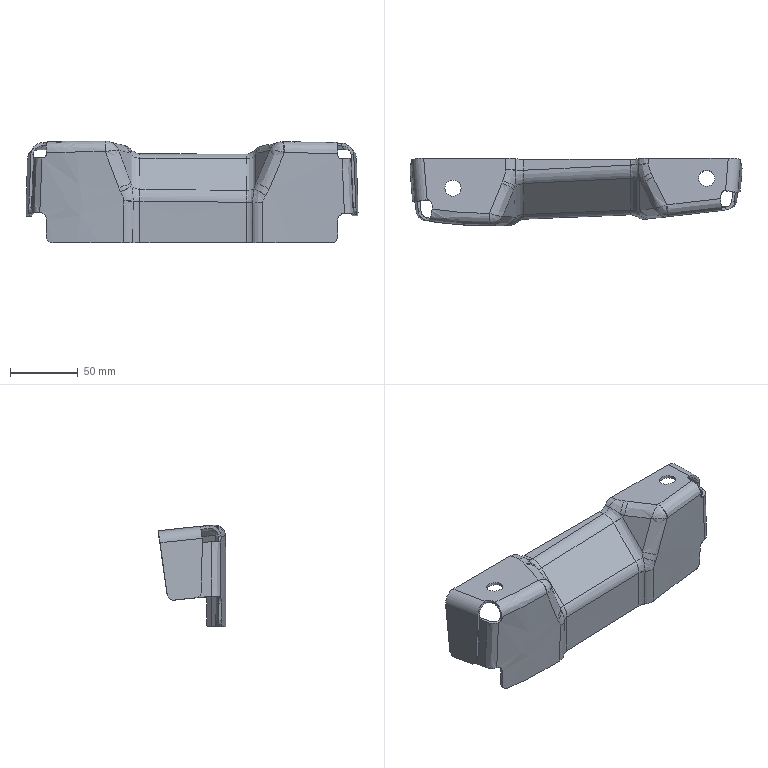Part | 1 solid | 194 faces | box 245.035 x 49.947 x 75.227 mm | volume 57937 mm3 | spline 137 | plane 35 | cylinder 18 | other 4 | commonest cylinder face diameters 10 x8 12 x4 14 x2 18 x2 20 x1 24 x1